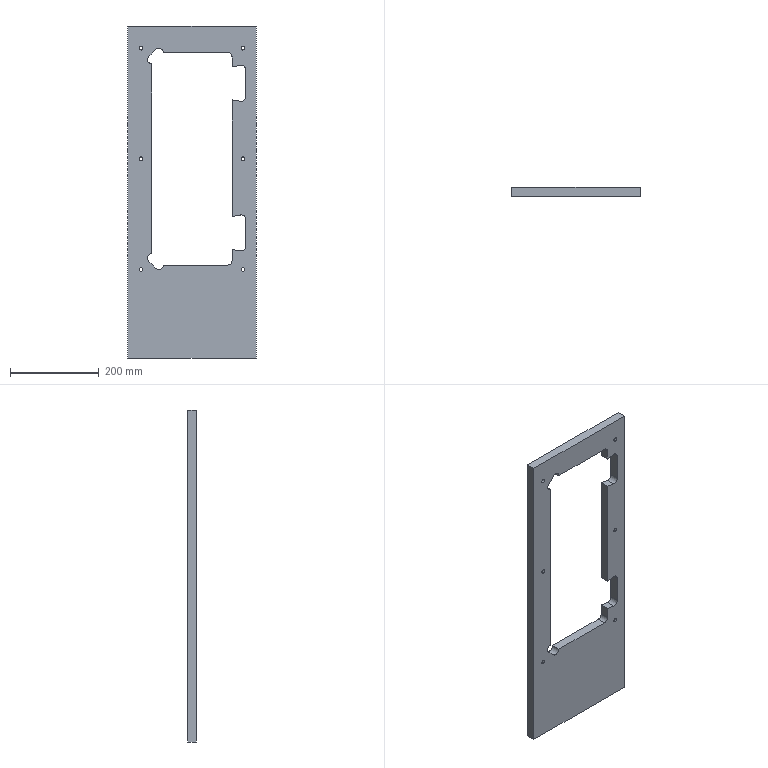Part | STEP file | A14-008 | 1 solid | 63 faces | box 290 x 20 x 750 mm | volume 2491365 mm3 | cylinder 37 | plane 26 | commonest cylinder face diameters 20 x13 8.5 x12 13.5 x12